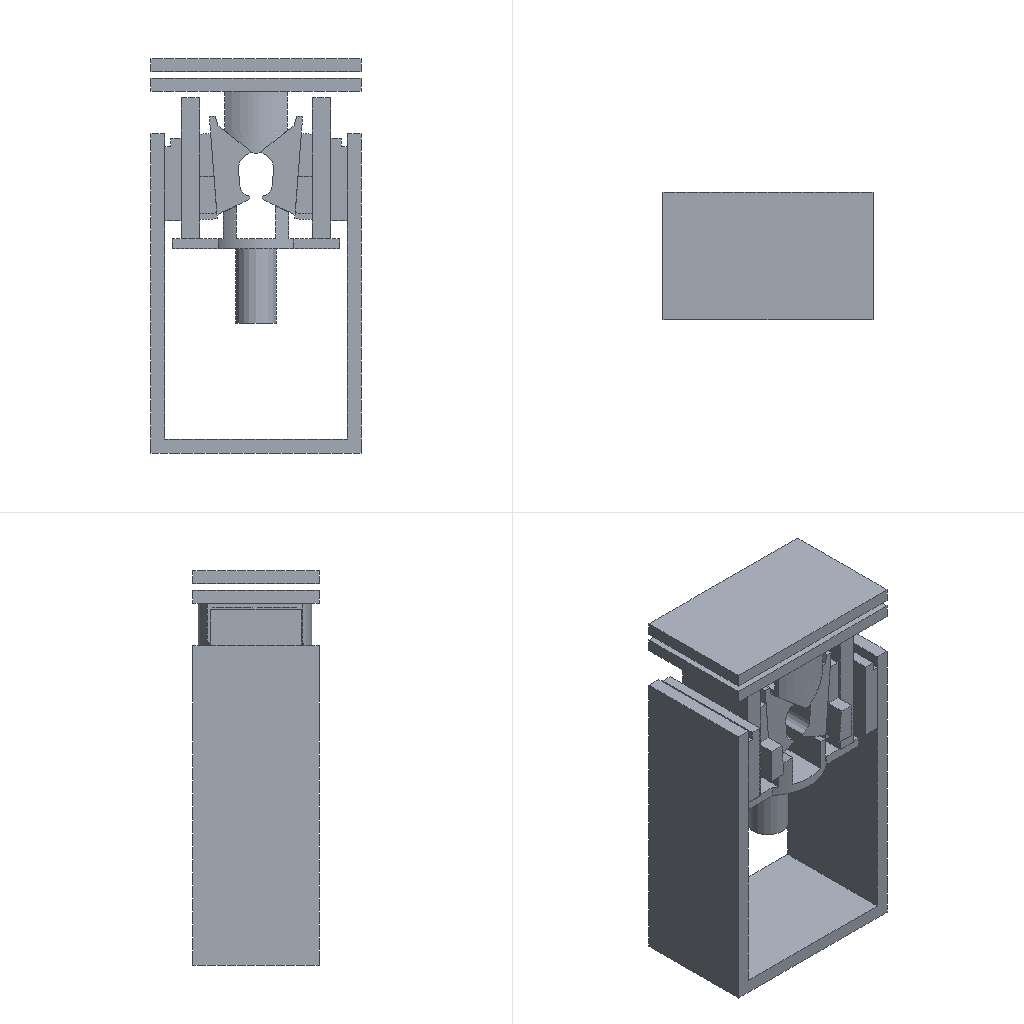Simulation study | abaqus
Set-up summary:
category,name,step,type,value,unit,region
solver,abaqus,,Abaqus/CAE 2024
units,mm-N-s-tonne (MPa),,inferred,E=212000 density=7.86e-09
analysis,Step-1,,dynamic temp-displacement,nlgeom=True; time_period=0.01
mesh,nodes,,,64430
mesh,elements,,,47881
element_type,C3D8T,,,47876
element_type,MASS,,,3
element_type,CONN3D2,,,2
material,hcq,,E,212000
material,hcq,,nu,0.3
material,hcq,,density,7.86e-09
material,hcq,,yield,400
material,hcq,,conductivity,50
material,hcq,,specific_heat,9.6e+08
material,hcq,,cte,1e-05
material,hcq,,behaviors,plastic; conductivity; expansion; specific heat
section,hcq,,solid section,,,Set-3
section,hcq,,solid section,,,Set-9
section,hcq,,solid section,,,Set-6
section,hcq,,solid section,,,Set-14
section,hcq,,solid section,,,Set-1
section,hcq,,solid section,,,Set-4
section,hcq,,solid section,,,Set-1
section,hcq,,solid section,,,Set-1
section,hcq,,solid section,,,Set-2
load,Predefined,initial,initial condition temperature
bc,BC-2,initial,encastre,[dofs=ENCASTRE],,Set-15
bc,BC-1,Step-1,velocity,"-2000 [dofs=x,y,z n=3]",,Set-5
contact,Constraint-2,initial,tie,,,s_Surf-17 / m_Surf-17
contact,Constraint-3,initial,tie,,,s_Surf-19 / m_Surf-19
contact,Constraint-4,initial,tie,,,s_Surf-21 / m_Surf-21
contact,Int-9,initial,general contact,interaction=IntProp-1; friction=0.3; behavior=hard
constraint,connector section,,,2
constraint,coupling,,,3
Abaqus input file, long lists of numbers shortened:
*Heading
** Job name: deck Model name: Model-1-Copy-Copy
** Generated by: Abaqus/CAE 2024
*Preprint, echo=NO, model=NO, history=NO, contact=NO
**
** PARTS
**
*Part, name=dongaban
*Node
      1,         -70.,        107.5,           0.
      2,         -70.,   99.537,           0.
** (2658 more lines like these left out)
*Element, type=C3D8T
   1,  141,  142,  170,  169,    1,    2,   30,   29
   2,  142,  143,  171,  170,    2,    3,   31,   30
** (1942 more lines like these left out)
*Nset, nset=Set-3, generate
    1,  2660,     1
*Elset, elset=Set-3, generate
    1,  1944,     1
** Section: Section-1
*Solid Section, elset=Set-3, material=hcq
,
*End Part
**
*Part, name=gudingxieban
*Node
      1,          94.,         -28.,         13.5
      2,          94.,         -28.,         24.5
** (6109 more lines like these left out)
*Element, type=C3D8T
  1,  214, 1306, 3776, 1084,    1,   55,  940,   68
  2, 1306, 1307, 3777, 3776,   55,   56,  941,  940
** (4846 more lines like these left out)
*Nset, nset=Set-9, generate
    1,  6111,     1
*Elset, elset=Set-9, generate
    1,  4848,     1
** Section: Section-1
*Solid Section, elset=Set-9, material=hcq
,
*End Part
**
*Part, name=tanhuangzuo
*Node
      1,   -83.442,           0.,          30.
      2,   -83.442,          15.,          30.
** (9119 more lines like these left out)
*Element, type=C3D8T
  1,  143, 1319, 5444, 1193,    1,   87, 1157,  108
  2, 1319, 1320, 5445, 5444,   87,   88, 1158, 1157
** (6650 more lines like these left out)
*Nset, nset=Set-6, generate
    1,  9121,     1
*Elset, elset=Set-6, generate
    1,  6652,     1
** Section: Section-1
*Solid Section, elset=Set-6, material=hcq
,
*End Part
**
*Part, name=waigudingban
*Node
      1,           7.,           0.,          18.
      2,           7.,         -35.,          18.
** (6070 more lines like these left out)
*Element, type=C3D8T
 1,  183, 1581, 1593,  182,    1,  157,  168,    4
 2, 1581, 1582, 1594, 1593,  157,  158,  167,  168
** (4610 more lines like these left out)
*Nset, nset=Set-14, generate
    1,  6072,     1
*Elset, elset=Set-14, generate
    1,  4612,     1
** Section: Section-1
*Solid Section, elset=Set-14, material=hcq
,
*End Part
**
*Part, name=xiangti
*Node
      1,         139.,        -96.5,          22.
      2,         139.,        -96.5,         487.
** (7618 more lines like these left out)
*Element, type=C3D8T
   1,  282, 2429, 5443, 2393,    1,   25,  737,  152
   2, 2429, 2430, 5444, 5443,   25,   26,  738,  737
** (4786 more lines like these left out)
*Node
   7621,           0.,           0.,          22.
*Nset, nset=xiangti-RefPt_, internal
7621,
*Nset, nset=Set-1, generate
    1,  7620,     1
*Elset, elset=Set-1, generate
    1,  4788,     1
** Section: Section-1
*Solid Section, elset=Set-1, material=hcq
,
*End Part
**
*Part, name=xiekuai
*Node
      1,           0.,           0.,         130.
      2,   19.199,  -50.074,         130.
** (4966 more lines like these left out)
*Element, type=C3D8T
   1,    3,    2,    5,    4,  219,  218,  221,  220
   2,    5,    2,   27,   75,  221,  218,  243,  291
** (3980 more lines like these left out)
*Nset, nset=Set-4, generate
    1,  4968,     1
*Elset, elset=Set-4, generate
    1,  3982,     1
** Section: Section-1
*Solid Section, elset=Set-4, material=hcq
,
*End Part
**
*Part, name=yali
*Node
      1,        -290.,         -20.,          20.
      2,        -290.,  -9.842,          20.
** (1978 more lines like these left out)
*Element, type=C3D8T
   1,   61,   62,   82,   81,    1,    2,   22,   21
   2,   62,   63,   83,   82,    2,    3,   23,   22
** (1214 more lines like these left out)
*Nset, nset=Set-1, generate
    1,  1980,     1
*Elset, elset=Set-1, generate
    1,  1216,     1
** Section: Section-1
*Solid Section, elset=Set-1, material=hcq
,
*End Part
**
*Part, name=yuyaban
*Node
      1,        -290.,         -20.,          20.
      2,        -290.,  -9.842,          20.
** (1978 more lines like these left out)
*Element, type=C3D8T
   1,   61,   62,   82,   81,    1,    2,   22,   21
   2,   62,   63,   83,   82,    2,    3,   23,   22
** (1214 more lines like these left out)
*Nset, nset=Set-1, generate
    1,  1980,     1
*Elset, elset=Set-1, generate
    1,  1216,     1
** Section: Section-1
*Solid Section, elset=Set-1, material=hcq
,
*End Part
**
*Part, name=zhongxinxiekuai
*Node
      1,         12.5,         72.5,          52.
      2,         12.5,         72.5,          60.
** (4102 more lines like these left out)
*Element, type=C3D8T
 1,    1,  109,  797,  114,  123,  809, 2369,  801
 2,  109,    2,  110,  797,  809,  127,  805, 2369
** (3230 more lines like these left out)
*Nset, nset=Set-2, generate
    1,  4104,     1
*Elset, elset=Set-2, generate
    1,  3232,     1
** Section: Section-1
*Solid Section, elset=Set-2, material=hcq
,
*End Part
**
**
** ASSEMBLY
**
*Assembly, name=Assembly
**
*Instance, name=zhongxinxiekuai, part=zhongxinxiekuai
12.272, 24.554, 794.895
12.272, 24.554, 794.895, 12.272, 25.554, 794.895,         180.
*End Instance
**
*Instance, name=xiekuai, part=xiekuai
-47.226, 87.606, 606.989
-47.226, 87.606, 606.989, -47.774, 88.197, 606.397, 237.425
*End Instance
**
*Instance, name=gudingxieban, part=gudingxieban
-75.15, 22.606, 636.723
-75.15, 22.606, 636.723, -75.72, 23.176, 636.131, 118.737
*End Instance
**
*Instance, name=dongban, part=dongaban
-101.728, 22.606,         678.
-101.728, 22.606,         678., -101.151, 23.183, 678.577,         120.
*End Instance
**
*Instance, name=xiekuai1, part=xiekuai
71.769, -42.394, 606.989
71.769, -42.394, 606.989, 71.162, -42.956, 606.427, 117.49
*End Instance
**
*Instance, name=waigudingban1, part=waigudingban
126.272, 22.606,        660.5
126.272, 22.606,        660.5, 125.694, 23.183, 659.923,         120.
*End Instance
**
*Instance, name=gudingxieban1, part=gudingxieban
72.714, 22.606, 637.761
72.714, 22.606, 637.761, 73.298, 22.021, 638.323, 238.72
*End Instance
**
*Instance, name=dongaban1, part=dongaban
98.272, 22.606,         678.
98.272, 22.606,         678., 98.849, 23.183, 678.577,         120.
*End Instance
**
*Instance, name=tanhuangzuo, part=tanhuangzuo
12.272, 22.606,        555.5
12.272, 22.606,        555.5, 12.849, 23.183, 556.077,         120.
*End Instance
**
*Instance, name=xiangti, part=xiangti
12.272, 22.606,        243.5
*End Instance
**
*Instance, name=waigudingban, part=waigudingban
-101.728, 22.606,        660.5
-101.728, 22.606,        660.5, -101.151, 23.183, 659.923,         240.
*End Instance
**
*Instance, name=yuyaban-1, part=yuyaban
142.272, -53.894, 794.895
*End Instance
**
*Instance, name=yali-1, part=yali
142.272, -53.894, 824.895
*End Instance
**
*Node
      1,   12.272,   22.606,   699.895
*Node
      2,   12.272,   22.606,        570.5
*Element, type=CONN3D2
4, 1, 2
*Connector Section, elset=_PickedSet114, behavior=ConnSect-2
Translator,
"Datum csys-2",
*Element, type=CONN3D2
5, 2, xiangti0.7621
*Connector Section, elset=_PickedSet117, behavior=ConnSect-1
Translator,
"Datum csys-2",
*Nset, nset=Set-1, instance=zhongxinxiekuai, generate
    1,  4104,     1
*Nset, nset=Set-1, instance=xiekuai, generate
    1,  4968,     1
*Nset, nset=Set-1, instance=dongban, generate
    1,  2660,     1
*Nset, nset=Set-1, instance=gudingxieban1, generate
    1,  6111,     1
*Nset, nset=Set-1, instance=xiekuai1, generate
    1,  4968,     1
*Nset, nset=Set-1, instance=tanhuangzuo, generate
    1,  9121,     1
*Nset, nset=Set-1, instance=gudingxieban, generate
    1,  6111,     1
*Nset, nset=Set-1, instance=dongaban1, generate
    1,  2660,     1
*Nset, nset=Set-1, instance=waigudingban1, generate
    1,  6072,     1
*Nset, nset=Set-1, instance=xiangti, generate
    1,  7620,     1
*Elset, elset=Set-1, instance=zhongxinxiekuai, generate
    1,  3232,     1
*Elset, elset=Set-1, instance=xiekuai, generate
    1,  3982,     1
*Elset, elset=Set-1, instance=dongban, generate
    1,  1944,     1
*Elset, elset=Set-1, instance=gudingxieban1, generate
    1,  4848,     1
*Elset, elset=Set-1, instance=xiekuai1, generate
    1,  3982,     1
*Elset, elset=Set-1, instance=tanhuangzuo, generate
    1,  6652,     1
*Elset, elset=Set-1, instance=gudingxieban, generate
    1,  4848,     1
*Elset, elset=Set-1, instance=dongaban1, generate
    1,  1944,     1
*Elset, elset=Set-1, instance=waigudingban1, generate
    1,  4612,     1
*Elset, elset=Set-1, instance=xiangti, generate
    1,  4788,     1
*Nset, nset=Set-4, instance=zhongxinxiekuai
   84,   85,   86,   87,   88,   89,   90,   91,   92,   93,   94,   95,   96,   98,   99,  100
  101,  102,  103,  104,  557,  558,  559,  560,  561,  562,  563,  567,  568,  569,  570,  571
** (15 more lines like these left out)
*Elset, elset=Set-4, instance=zhongxinxiekuai
 1032, 1033, 1034, 1035, 1036, 1037, 1038, 1039, 1048, 1049, 1050, 1051, 1052, 1053, 1054, 1055
 1064, 1065, 1066, 1067, 1068, 1069, 1070, 1071, 1072, 1073, 1074, 1075, 1076, 1077, 1078, 1079
** (13 more lines like these left out)
*Nset, nset=Set-5, instance=yali-1
    1,    2,    3,    4,    5,    6,    7,    8,    9,   10,   11,   12,   13,   14,   15,   16
   17,   18,   19,   20,   61,   62,   63,   64,   65,   66,   67,   68,   69,   70,   71,   72
** (40 more lines like these left out)
*Elset, elset=Set-5, instance=yali-1
    1,    2,    3,    4,    5,    6,    7,    8,    9,   10,   11,   12,   13,   14,   15,   16
   17,   18,   19,   39,   40,   41,   42,   43,   44,   45,   46,   47,   48,   49,   50,   51
** (36 more lines like these left out)
*Nset, nset=Set-7, instance=zhongxinxiekuai, generate
    1,  4104,     1
*Nset, nset=Set-7, instance=xiekuai, generate
    1,  4968,     1
*Nset, nset=Set-7, instance=dongban, generate
    1,  2660,     1
*Nset, nset=Set-7, instance=gudingxieban1, generate
    1,  6111,     1
*Nset, nset=Set-7, instance=xiekuai1, generate
    1,  4968,     1
*Nset, nset=Set-7, instance=tanhuangzuo, generate
    1,  9121,     1
*Nset, nset=Set-7, instance=yali-1, generate
    1,  1980,     1
*Nset, nset=Set-7, instance=gudingxieban, generate
    1,  6111,     1
*Nset, nset=Set-7, instance=dongaban1, generate
    1,  2660,     1
*Nset, nset=Set-7, instance=waigudingban1, generate
    1,  6072,     1
*Nset, nset=Set-7, instance=xiangti, generate
    1,  7620,     1
*Nset, nset=Set-7, instance=yuyaban-1, generate
    1,  1980,     1
*Nset, nset=Set-7, instance=waigudingban, generate
    1,  6072,     1
*Elset, elset=Set-7, instance=zhongxinxiekuai, generate
    1,  3232,     1
*Elset, elset=Set-7, instance=xiekuai, generate
    1,  3982,     1
*Elset, elset=Set-7, instance=dongban, generate
    1,  1944,     1
*Elset, elset=Set-7, instance=gudingxieban1, generate
    1,  4848,     1
*Elset, elset=Set-7, instance=xiekuai1, generate
    1,  3982,     1
*Elset, elset=Set-7, instance=tanhuangzuo, generate
    1,  6652,     1
*Elset, elset=Set-7, instance=yali-1, generate
    1,  1216,     1
*Elset, elset=Set-7, instance=gudingxieban, generate
    1,  4848,     1
*Elset, elset=Set-7, instance=dongaban1, generate
    1,  1944,     1
*Elset, elset=Set-7, instance=waigudingban1, generate
    1,  4612,     1
*Elset, elset=Set-7, instance=xiangti, generate
    1,  4788,     1
*Elset, elset=Set-7, instance=yuyaban-1, generate
    1,  1216,     1
*Elset, elset=Set-7, instance=waigudingban, generate
    1,  4612,     1
*Nset, nset=Set-15, instance=xiangti
    5,    6,    7,    8,    9,   10,   11,   12,   15,   16,   17,   18,   19,   20,   21,   22
  153,  154,  155,  156,  157,  158,  159,  160,  161,  162,  163,  164,  165,  166,  167,  168
** (162 more lines like these left out)
*Elset, elset=Set-15, instance=xiangti
  894,  895,  896,  897,  898,  899,  900,  901,  902,  903,  904,  905,  906,  907,  908,  909
  910,  911,  912,  913,  914,  915,  916,  917,  918,  919,  920,  921,  922,  923,  924,  925
** (150 more lines like these left out)
*Nset, nset=Set-16, instance=zhongxinxiekuai, generate
    1,  4104,     1
*Nset, nset=Set-16, instance=xiekuai, generate
    1,  4968,     1
*Nset, nset=Set-16, instance=dongban, generate
    1,  2660,     1
*Nset, nset=Set-16, instance=gudingxieban1, generate
    1,  6111,     1
*Nset, nset=Set-16, instance=xiekuai1, generate
    1,  4968,     1
*Nset, nset=Set-16, instance=tanhuangzuo, generate
    1,  9121,     1
*Nset, nset=Set-16, instance=yali-1, generate
    1,  1980,     1
*Nset, nset=Set-16, instance=gudingxieban, generate
    1,  6111,     1
*Nset, nset=Set-16, instance=dongaban1, generate
    1,  2660,     1
*Nset, nset=Set-16, instance=waigudingban1, generate
    1,  6072,     1
*Nset, nset=Set-16, instance=xiangti, generate
    1,  7620,     1
*Nset, nset=Set-16, instance=yuyaban-1, generate
    1,  1980,     1
*Nset, nset=Set-16, instance=waigudingban, generate
    1,  6072,     1
*Elset, elset=Set-16, instance=zhongxinxiekuai, generate
    1,  3232,     1
*Elset, elset=Set-16, instance=xiekuai, generate
    1,  3982,     1
*Elset, elset=Set-16, instance=dongban, generate
    1,  1944,     1
*Elset, elset=Set-16, instance=gudingxieban1, generate
    1,  4848,     1
*Elset, elset=Set-16, instance=xiekuai1, generate
    1,  3982,     1
*Elset, elset=Set-16, instance=tanhuangzuo, generate
    1,  6652,     1
*Elset, elset=Set-16, instance=yali-1, generate
    1,  1216,     1
*Elset, elset=Set-16, instance=gudingxieban, generate
    1,  4848,     1
*Elset, elset=Set-16, instance=dongaban1, generate
    1,  1944,     1
*Elset, elset=Set-16, instance=waigudingban1, generate
    1,  4612,     1
*Elset, elset=Set-16, instance=xiangti, generate
    1,  4788,     1
*Elset, elset=Set-16, instance=yuyaban-1, generate
    1,  1216,     1
*Elset, elset=Set-16, instance=waigudingban, generate
    1,  4612,     1
*Nset, nset=Wire-1-Set-1
 1, 2
*Elset, elset=Wire-1-Set-1
 4,
*Nset, nset=Wire-2-Set-1
 2,
*Nset, nset=Wire-2-Set-1, instance=xiangti
 7621,
*Elset, elset=Wire-2-Set-1
 5,
*Nset, nset=b_Set-2, instance=xiangti, generate
    1,  7620,     1
*Elset, elset=b_Set-2, instance=xiangti, generate
    1,  4788,     1
*Nset, nset=m_Set-6, instance=zhongxinxiekuai, generate
   1,  108,    1
*Nset, nset=m_Set-6, instance=xiekuai
    1,    2,    5,    8,    9,   13,   16,   17,   18,   19, 4753, 4754, 4757, 4760, 4761, 4765
 4768, 4769, 4770, 4771
*Nset, nset=m_Set-6, instance=dongban
    1,   28,  113,  140, 2521, 2548, 2633, 2660
*Nset, nset=m_Set-6, instance=gudingxieban1, generate
  1,  54,   1
*Nset, nset=m_Set-6, instance=xiekuai1
    1,    2,    5,    8,    9,   13,   16,   17,   18,   19, 4753, 4754, 4757, 4760, 4761, 4765
 4768, 4769, 4770, 4771
*Nset, nset=m_Set-6, instance=tanhuangzuo, generate
  1,  86,   1
*Nset, nset=m_Set-6, instance=yali-1
    1,   20,   41,   60, 1921, 1940, 1961, 1980
*Nset, nset=m_Set-6, instance=gudingxieban, generate
  1,  54,   1
*Nset, nset=m_Set-6, instance=dongaban1
    1,   28,  113,  140, 2521, 2548, 2633, 2660
*Nset, nset=m_Set-6, instance=waigudingban1, generate
   1,  156,    1
*Nset, nset=m_Set-6, instance=xiangti, generate
  1,  24,   1
*Nset, nset=m_Set-6, instance=yuyaban-1
    1,   20,   41,   60, 1921, 1940, 1961, 1980
*Nset, nset=m_Set-6, instance=waigudingban, generate
   1,  156,    1
*Nset, nset=m_Set-12, instance=xiangti
 7621,
*Nset, nset=m_Set-13
 2,
*Nset, nset=m_Set-15
 1,
*Nset, nset=s_Set-13, instance=tanhuangzuo
  5,  8,  9, 10, 14, 18, 57, 62
*Elset, elset=_PickedSet114, internal
 4,
*Elset, elset=_PickedSet117, internal
 5,
*Elset, elset=_m_Surf-1_S5, internal, instance=dongaban1
   82,   83,   84,   85,   86,   87,   88,   89,   90,   91,   92,   93,   94,   95,   96,   97
   98,   99,  100,  101,  102,  103,  104,  105,  106,  107,  108,  190,  191,  192,  193,  194
** (29 more lines like these left out)
*Surface, type=ELEMENT, name=m_Surf-1
_m_Surf-1_S5, S5
*Elset, elset=_m_Surf-3_S3, internal, instance=dongaban1
    1,    2,    3,    4,    5,    6,    7,    8,    9,   10,   11,   12,   13,   14,   15,   16
   17,   18,   19,   20,   21,   22,   23,   24,   25,   26,   27,  109,  110,  111,  112,  113
** (29 more lines like these left out)
*Surface, type=ELEMENT, name=m_Surf-3
_m_Surf-3_S3, S3
*Elset, elset=_m_Surf-5_S3, internal, instance=dongban
    1,    2,    3,    4,    5,    6,    7,    8,    9,   10,   11,   12,   13,   14,   15,   16
   17,   18,   19,   20,   21,   22,   23,   24,   25,   26,   27,  109,  110,  111,  112,  113
** (29 more lines like these left out)
*Surface, type=ELEMENT, name=m_Surf-5
_m_Surf-5_S3, S3
*Elset, elset=_m_Surf-7_S5, internal, instance=dongban
   82,   83,   84,   85,   86,   87,   88,   89,   90,   91,   92,   93,   94,   95,   96,   97
   98,   99,  100,  101,  102,  103,  104,  105,  106,  107,  108,  190,  191,  192,  193,  194
** (29 more lines like these left out)
*Surface, type=ELEMENT, name=m_Surf-7
_m_Surf-7_S5, S5
*Elset, elset=_m_Surf-9_S5, internal, instance=xiekuai1
    4,    6,   20,   21,   26,   33,   35,   38,   41,   53,   57,  185,  187,  201,  202,  207
  214,  216,  219,  222,  234,  238,  366,  368,  382,  383,  388,  395,  397,  400,  403,  415
** (14 more lines like these left out)
*Elset, elset=_m_Surf-9_S3, internal, instance=xiekuai1
    5,   28,   30,   31,   36,   42,   44,   46,   49,   61,   64,   71,   73,   76,  186,  209
  211,  212,  217,  223,  225,  227,  230,  242,  245,  252,  254,  257,  367,  390,  392,  393
** (18 more lines like these left out)
*Surface, type=ELEMENT, name=m_Surf-9
_m_Surf-9_S5, S5
_m_Surf-9_S3, S3
*Elset, elset=_m_Surf-11_S4, internal, instance=xiekuai1
    9,   22,   68,   83,   84,  190,  203,  249,  264,  265,  371,  384,  430,  445,  446,  552
  565,  611,  626,  627,  733,  746,  792,  807,  808,  914,  927,  973,  988,  989, 1095, 1108
** (5 more lines like these left out)
*Elset, elset=_m_Surf-11_S3, internal, instance=xiekuai1, generate
   23,  3824,   181
*Elset, elset=_m_Surf-11_S6, internal, instance=xiekuai1
   25,   69,   70,   91,  206,  250,  251,  272,  387,  431,  432,  453,  568,  612,  613,  634
  749,  793,  794,  815,  930,  974,  975,  996, 1111, 1155, 1156, 1177, 1292, 1336, 1337, 1358
** (4 more lines like these left out)
*Surface, type=ELEMENT, name=m_Surf-11
_m_Surf-11_S4, S4
_m_Surf-11_S3, S3
_m_Surf-11_S6, S6
*Elset, elset=_m_Surf-13_S3, internal, instance=zhongxinxiekuai
 1582, 1662, 1666, 1670, 1674, 1678, 1682, 1686, 1819, 1899, 1903, 1907, 1911, 1915, 1919, 1923
 2056, 2136, 2140, 2144, 2148, 2152, 2156, 2160, 2293, 2373, 2377, 2381, 2385, 2389, 2393, 2397
** (2 more lines like these left out)
*Elset, elset=_m_Surf-13_S5, internal, instance=zhongxinxiekuai
 1690, 1697, 1701, 1705, 1709, 1713, 1717, 1721, 1725, 1927, 1934, 1938, 1942, 1946, 1950, 1954
 1958, 1962, 2164, 2171, 2175, 2179, 2183, 2187, 2191, 2195, 2199, 2401, 2408, 2412, 2416, 2420
** (2 more lines like these left out)
*Surface, type=ELEMENT, name=m_Surf-13
_m_Surf-13_S3, S3
_m_Surf-13_S5, S5
*Elset, elset=_m_Surf-15_S5, internal, instance=xiekuai
    4,    6,   20,   21,   26,   33,   35,   38,   41,   53,   57,  185,  187,  201,  202,  207
  214,  216,  219,  222,  234,  238,  366,  368,  382,  383,  388,  395,  397,  400,  403,  415
** (14 more lines like these left out)
*Elset, elset=_m_Surf-15_S3, internal, instance=xiekuai
    5,   28,   30,   31,   36,   42,   44,   46,   49,   61,   64,   71,   73,   76,  186,  209
  211,  212,  217,  223,  225,  227,  230,  242,  245,  252,  254,  257,  367,  390,  392,  393
** (18 more lines like these left out)
*Surface, type=ELEMENT, name=m_Surf-15
_m_Surf-15_S5, S5
_m_Surf-15_S3, S3
*Elset, elset=_m_Surf-17_S5, internal, instance=yuyaban-1
   20,   21,   22,   23,   24,   25,   26,   27,   28,   29,   30,   31,   32,   33,   34,   35
   36,   37,   38,   58,   59,   60,   61,   62,   63,   64,   65,   66,   67,   68,   69,   70
** (36 more lines like these left out)
*Surface, type=ELEMENT, name=m_Surf-17
_m_Surf-17_S5, S5
*Elset, elset=_m_Surf-19_S1, internal, instance=xiangti, generate
 3896,  4788,     1
*Surface, type=ELEMENT, name=m_Surf-19
_m_Surf-19_S1, S1
*Elset, elset=_m_Surf-21_S2, internal, instance=xiangti, generate
   1,  893,    1
*Surface, type=ELEMENT, name=m_Surf-21
_m_Surf-21_S2, S2
*Elset, elset=_s_Surf-1_S5, internal, instance=waigudingban1
  262,  263,  264,  271,  272,  273,  280,  281,  282,  996,  997,  998, 1005, 1006, 1007, 1014
 1015, 1016, 1023, 1024, 1025, 1032, 1033, 1034, 1041, 1042, 1043, 1050, 1051, 1052, 1059, 1060
** (11 more lines like these left out)
*Elset, elset=_s_Surf-1_S6, internal, instance=waigudingban1
   49,   52,   55,   58,   61,   64,   67,   70,   73,   76,   79,   82,   85,   88,   91,   94
   97,  100,  103,  106,  109,  112,  115,  118,  121,  124,  127,  130,  133,  136,  139,  142
** (27 more lines like these left out)
*Elset, elset=_s_Surf-1_S4, internal, instance=waigudingban1
 1373, 1376, 1379, 1382, 1385, 1388, 1391, 1394, 1397, 1400, 1403, 1406, 1409, 1412, 1415, 1418
 1421, 1424, 1427, 1430, 1433, 1436, 1439, 1442, 1445, 1448, 1451, 1454, 1457, 1460, 1883, 1886
** (21 more lines like these left out)
*Surface, type=ELEMENT, name=s_Surf-1
_s_Surf-1_S5, S5
_s_Surf-1_S6, S6
_s_Surf-1_S4, S4
*Elset, elset=_s_Surf-3_S4, internal, instance=gudingxieban1
    3,    6,    9,   12,   15,   18,   21,   24,   27,   30,   33,   36,   39,   42,   45,   48
   51,   54,   57,   60,   63,   66,   69,   72,   75,   78,   81,   84,   87,   90,   93,   96
** (13 more lines like these left out)
*Elset, elset=_s_Surf-3_S6, internal, instance=gudingxieban1, generate
 3781,  4006,     3
*Elset, elset=_s_Surf-3_S5, internal, instance=gudingxieban1
 1601, 1602, 1607, 1608, 1613, 1614, 1619, 1620, 1625, 1626, 1631, 1632, 1637, 1638, 1643, 1644
 1649, 1650, 1655, 1656, 1661, 1662, 1667, 1668, 1673, 1674, 1679, 1680, 1685, 1686, 1691, 1692
** (30 more lines like these left out)
*Surface, type=ELEMENT, name=s_Surf-3
_s_Surf-3_S4, S4
_s_Surf-3_S6, S6
_s_Surf-3_S5, S5
*Elset, elset=_s_Surf-5_S5, internal, instance=waigudingban
  262,  263,  264,  271,  272,  273,  280,  281,  282,  996,  997,  998, 1005, 1006, 1007, 1014
 1015, 1016, 1023, 1024, 1025, 1032, 1033, 1034, 1041, 1042, 1043, 1050, 1051, 1052, 1059, 1060
** (11 more lines like these left out)
*Elset, elset=_s_Surf-5_S6, internal, instance=waigudingban
   49,   52,   55,   58,   61,   64,   67,   70,   73,   76,   79,   82,   85,   88,   91,   94
   97,  100,  103,  106,  109,  112,  115,  118,  121,  124,  127,  130,  133,  136,  139,  142
** (27 more lines like these left out)
*Elset, elset=_s_Surf-5_S4, internal, instance=waigudingban
 1373, 1376, 1379, 1382, 1385, 1388, 1391, 1394, 1397, 1400, 1403, 1406, 1409, 1412, 1415, 1418
 1421, 1424, 1427, 1430, 1433, 1436, 1439, 1442, 1445, 1448, 1451, 1454, 1457, 1460, 1883, 1886
** (21 more lines like these left out)
*Surface, type=ELEMENT, name=s_Surf-5
_s_Surf-5_S5, S5
_s_Surf-5_S6, S6
_s_Surf-5_S4, S4
*Elset, elset=_s_Surf-7_S5, internal, instance=gudingxieban
  465,  466,  467,  468,  477,  478,  479,  480,  489,  490,  491,  492,  501,  502,  503,  504
  513,  514,  515,  516,  525,  526,  527,  528,  537,  538,  539,  540,  549,  550,  551,  552
** (36 more lines like these left out)
*Elset, elset=_s_Surf-7_S2, internal, instance=gudingxieban
 1141, 1142, 1143, 1144, 1145, 1146, 1147, 1148, 1149, 1150, 1151, 1152, 1153, 1154, 1155, 1156
 1157, 1158, 1159, 1160, 1161, 1162, 1163, 1164, 1165, 1166, 1167, 1168, 1169, 1170, 1171, 1172
** (11 more lines like these left out)
*Surface, type=ELEMENT, name=s_Surf-7
_s_Surf-7_S5, S5
_s_Surf-7_S2, S2
*Elset, elset=_s_Surf-9_S5, internal, instance=gudingxieban1
  465,  466,  467,  468,  477,  478,  479,  480,  489,  490,  491,  492,  501,  502,  503,  504
  513,  514,  515,  516,  525,  526,  527,  528,  537,  538,  539,  540,  549,  550,  551,  552
** (36 more lines like these left out)
*Elset, elset=_s_Surf-9_S2, internal, instance=gudingxieban1
 1141, 1142, 1143, 1144, 1145, 1146, 1147, 1148, 1149, 1150, 1151, 1152, 1153, 1154, 1155, 1156
 1157, 1158, 1159, 1160, 1161, 1162, 1163, 1164, 1165, 1166, 1167, 1168, 1169, 1170, 1171, 1172
** (11 more lines like these left out)
*Surface, type=ELEMENT, name=s_Surf-9
_s_Surf-9_S5, S5
_s_Surf-9_S2, S2
*Elset, elset=_s_Surf-11_S4, internal, instance=zhongxinxiekuai
 1609, 1753, 1757, 1761, 1765, 1769, 1773, 1777, 1785, 1846, 1990, 1994, 1998, 2002, 2006, 2010
 2014, 2022, 2083, 2227, 2231, 2235, 2239, 2243, 2247, 2251, 2259, 2320, 2464, 2468, 2472, 2476
** (2 more lines like these left out)
*Elset, elset=_s_Surf-11_S6, internal, instance=zhongxinxiekuai
 1631, 1632, 1633, 1634, 1635, 1636, 1637, 1868, 1869, 1870, 1871, 1872, 1873, 1874, 2105, 2106
 2107, 2108, 2109, 2110, 2111, 2342, 2343, 2344, 2345, 2346, 2347, 2348, 2579, 2580, 2581, 2582
** (2 more lines like these left out)
*Elset, elset=_s_Surf-11_S3, internal, instance=zhongxinxiekuai, generate
 1778,  3200,   237
*Surface, type=ELEMENT, name=s_Surf-11
_s_Surf-11_S4, S4
_s_Surf-11_S6, S6
_s_Surf-11_S3, S3
*Elset, elset=_s_Surf-13_S4, internal, instance=xiekuai
    9,   22,   68,   83,   84,  190,  203,  249,  264,  265,  371,  384,  430,  445,  446,  552
  565,  611,  626,  627,  733,  746,  792,  807,  808,  914,  927,  973,  988,  989, 1095, 1108
** (5 more lines like these left out)
*Elset, elset=_s_Surf-13_S3, internal, instance=xiekuai, generate
   23,  3824,   181
*Elset, elset=_s_Surf-13_S6, internal, instance=xiekuai
   25,   69,   70,   91,  206,  250,  251,  272,  387,  431,  432,  453,  568,  612,  613,  634
  749,  793,  794,  815,  930,  974,  975,  996, 1111, 1155, 1156, 1177, 1292, 1336, 1337, 1358
** (4 more lines like these left out)
*Surface, type=ELEMENT, name=s_Surf-13
_s_Surf-13_S4, S4
_s_Surf-13_S3, S3
_s_Surf-13_S6, S6
*Elset, elset=_s_Surf-15_S4, internal, instance=gudingxieban
    3,    6,    9,   12,   15,   18,   21,   24,   27,   30,   33,   36,   39,   42,   45,   48
   51,   54,   57,   60,   63,   66,   69,   72,   75,   78,   81,   84,   87,   90,   93,   96
** (13 more lines like these left out)
*Elset, elset=_s_Surf-15_S6, internal, instance=gudingxieban, generate
 3781,  4006,     3
*Elset, elset=_s_Surf-15_S5, internal, instance=gudingxieban
 1601, 1602, 1607, 1608, 1613, 1614, 1619, 1620, 1625, 1626, 1631, 1632, 1637, 1638, 1643, 1644
 1649, 1650, 1655, 1656, 1661, 1662, 1667, 1668, 1673, 1674, 1679, 1680, 1685, 1686, 1691, 1692
** (30 more lines like these left out)
*Surface, type=ELEMENT, name=s_Surf-15
_s_Surf-15_S4, S4
_s_Surf-15_S6, S6
_s_Surf-15_S5, S5
*Elset, elset=_s_Surf-17_S3, internal, instance=zhongxinxiekuai
 1032, 1033, 1048, 1049, 1050, 1051, 1064, 1065, 1066, 1067, 1408, 1409
*Elset, elset=_s_Surf-17_S4, internal, instance=zhongxinxiekuai
 1034, 1035, 1036, 1037, 1052, 1053, 1068, 1069, 1155, 1157, 1159, 1161, 1163, 1165, 1167, 1169
 1171, 1173, 1175, 1177, 1179, 1181, 1183, 1185, 1187, 1189, 1191, 1193, 1195, 1197, 1199, 1201
** (3 more lines like these left out)
*Elset, elset=_s_Surf-17_S2, internal, instance=zhongxinxiekuai
 1038, 1039, 1054, 1055, 1070, 1071, 1072, 1073, 1074, 1075, 1076, 1077, 1078, 1079, 1080, 1202
 1203, 1204, 1205, 1206, 1207, 1208, 1209, 1210, 1211, 1212, 1213, 1214, 1215, 1216, 1217, 1218
** (4 more lines like these left out)
*Elset, elset=_s_Surf-17_S6, internal, instance=zhongxinxiekuai
 1090, 1092, 1094, 1096, 1098, 1100, 1102, 1104, 1106, 1108, 1110, 1112, 1114, 1116, 1118, 1120
 1122, 1124, 1126, 1128, 1130, 1132, 1134, 1136, 1138, 1140, 1142, 1144, 1146, 1148, 1150, 1152
** (2 more lines like these left out)
*Surface, type=ELEMENT, name=s_Surf-17
_s_Surf-17_S3, S3
_s_Surf-17_S4, S4
_s_Surf-17_S2, S2
_s_Surf-17_S6, S6
*Elset, elset=_s_Surf-19_S6, internal, instance=waigudingban
  292,  293,  294,  295,  296,  297,  298,  299,  300, 1086, 1087, 1088, 1089, 1090, 1091, 1092
 1093, 1094, 1095, 1096, 1097, 1098, 1099, 1100, 1101, 1102, 1103, 1104, 1105, 1106, 1107, 1108
** (6 more lines like these left out)
*Elset, elset=_s_Surf-19_S3, internal, instance=waigudingban
  301,  302,  303,  304,  305,  306,  307,  308,  309, 1110, 1111, 1112, 1113, 1114, 1115, 1116
 1117, 1118, 1119, 1120, 1121, 1122, 1123, 1124, 1125, 1126, 1127, 1128, 1129, 1130, 1131, 1132
** (3 more lines like these left out)
*Elset, elset=_s_Surf-19_S5, internal, instance=waigudingban
   31,   32,   33,   34,   35,   36,   37,   38,   39,  390,  391,  392,  393,  394,  395,  396
  397,  398,  399,  400,  401,  402,  403,  404,  405,  406,  407,  408,  409,  410,  411,  412
** (22 more lines like these left out)
*Elset, elset=_s_Surf-19_S4, internal, instance=waigudingban, generate
 2181,  2210,     1
*Elset, elset=_s_Surf-19_S2, internal, instance=waigudingban, generate
 4361,  4430,     1
*Surface, type=ELEMENT, name=s_Surf-19
_s_Surf-19_S6, S6
_s_Surf-19_S3, S3
_s_Surf-19_S4, S4
_s_Surf-19_S2, S2
_s_Surf-19_S5, S5
*Elset, elset=_s_Surf-21_S6, internal, instance=waigudingban1
  292,  293,  294,  295,  296,  297,  298,  299,  300, 1086, 1087, 1088, 1089, 1090, 1091, 1092
 1093, 1094, 1095, 1096, 1097, 1098, 1099, 1100, 1101, 1102, 1103, 1104, 1105, 1106, 1107, 1108
** (6 more lines like these left out)
*Elset, elset=_s_Surf-21_S3, internal, instance=waigudingban1
  301,  302,  303,  304,  305,  306,  307,  308,  309, 1110, 1111, 1112, 1113, 1114, 1115, 1116
 1117, 1118, 1119, 1120, 1121, 1122, 1123, 1124, 1125, 1126, 1127, 1128, 1129, 1130, 1131, 1132
** (3 more lines like these left out)
*Elset, elset=_s_Surf-21_S5, internal, instance=waigudingban1
   31,   32,   33,   34,   35,   36,   37,   38,   39,  390,  391,  392,  393,  394,  395,  396
  397,  398,  399,  400,  401,  402,  403,  404,  405,  406,  407,  408,  409,  410,  411,  412
** (22 more lines like these left out)
*Elset, elset=_s_Surf-21_S4, internal, instance=waigudingban1, generate
 2181,  2210,     1
*Elset, elset=_s_Surf-21_S2, internal, instance=waigudingban1, generate
 4361,  4430,     1
*Surface, type=ELEMENT, name=s_Surf-21
_s_Surf-21_S6, S6
_s_Surf-21_S3, S3
_s_Surf-21_S4, S4
_s_Surf-21_S2, S2
_s_Surf-21_S5, S5
*Elset, elset=_s_Surf-23_S1, internal, instance=xiangti, generate
 2395,  2926,     1
*Surface, type=ELEMENT, name=s_Surf-23
_s_Surf-23_S1, S1
*Elset, elset=_s_Surf-24_S2, internal, instance=xiangti, generate
 1863,  2394,     1
*Surface, type=ELEMENT, name=s_Surf-24
_s_Surf-24_S2, S2
*Elset, elset=_s_Surf-25_S2, internal, instance=zhongxinxiekuai, generate
 2996,  3232,     1
*Surface, type=ELEMENT, name=s_Surf-25
_s_Surf-25_S2, S2
*Surface, type=NODE, name=s_Set-13_CNS_, internal
s_Set-13, 1.
*Orientation, name="Datum csys-2"
          0.,           0.,           1.,           0.,           1.,           0.
1, 0.
** Constraint: Constraint-2
*Tie, name=Constraint-2, adjust=no
s_Surf-17, m_Surf-17
** Constraint: Constraint-3
*Tie, name=Constraint-3, adjust=no
s_Surf-19, m_Surf-19
** Constraint: Constraint-4
*Tie, name=Constraint-4, adjust=no
s_Surf-21, m_Surf-21
** Constraint: Constraint-5
*Coupling, constraint name=Constraint-5, ref node=m_Set-12, surface=s_Surf-24
*Kinematic
** Constraint: Constraint-6
*Coupling, constraint name=Constraint-6, ref node=m_Set-13, surface=s_Set-13_CNS_
*Kinematic
** Constraint: Constraint-7
*Coupling, constraint name=Constraint-7, ref node=m_Set-15, surface=s_Surf-25
*Kinematic
*Element, type=MASS, elset=_PickedSet110_Inertia-1_
1, xiangti0.7621
2, 1
** (1 more lines like these left out)
*Mass, elset=_PickedSet110_Inertia-1_
1e-06,
*End Assembly
*Connector Behavior, name=ConnSect-2
*Connector Elasticity, component=1
129.,
*Connector Behavior, name=ConnSect-1
*Connector Elasticity, component=1
1287.,
**
** MATERIALS
**
*Material, name=hcq
*Conductivity
50.,
*Density
 7.86e-09,
*Elastic
212000., 0.3
*Expansion
 1e-05,
*Plastic
400.,0.
*Specific Heat
 9.6e+08,
**
** INTERACTION PROPERTIES
**
*Surface Interaction, name=IntProp-1
*Friction
 0.3,
*Surface Behavior, pressure-overclosure=HARD
*Gap Heat Generation
1., 0.5
*Surface Interaction, name=IntProp-2
*Friction
 0.3,
*Surface Behavior, pressure-overclosure=HARD
**
** BOUNDARY CONDITIONS
**
** Name: BC-2 Type: Symmetry/Antisymmetry/Encastre
*Boundary
Set-15, ENCASTRE
**
** PREDEFINED FIELDS
**
** Name: Predefined Field-1   Type: Temperature
*Initial Conditions, type=TEMPERATURE
Set-16, 25.
**
** INTERACTIONS
**
** Interaction: Int-9
*Contact, op=NEW
*Contact Inclusions, ALL EXTERIOR
*Contact Property Assignment
 ,  , IntProp-1
** ----------------------------------------------------------------
**
** STEP: Step-1
**
*Step, name=Step-1, nlgeom=YES
*Dynamic Temperature-displacement, Explicit
, 0.01
*Bulk Viscosity
0.06, 1.2
** Mass Scaling: Semi-Automatic
**               Whole Model
*Fixed Mass Scaling, factor=1000.
**
** BOUNDARY CONDITIONS
**
** Name: BC-1 Type: Velocity/Angular velocity
*Boundary, type=VELOCITY
Set-5, 1, 1
Set-5, 2, 2
Set-5, 3, 3, -2000.
**
** OUTPUT REQUESTS
**
*Restart, write, number interval=1, time marks=NO
**
** FIELD OUTPUT: F-Output-1
**
*Output, field
*Node Output
A, NT, RF, RFL, U, V
*Element Output, directions=YES
EVF, HFL, LE, PE, PEEQ, PEEQVAVG, PEVAVG, S, SVAVG, TEMP
*Contact Output
CSTRESS,
**
** HISTORY OUTPUT: H-Output-1
**
*Output, history, variable=PRESELECT, frequency=1
*End Step
Results summary:
result,odb.job_status,,,JOB_STATUS_COMPLETED_SUCCESSFULLY,"consistent, unstated (Abaqus has no unit system)"
result,steps[0].procedure,Step-1,,"*DYNAMIC TEMPERATURE-DISPLACEMENT, EXPLICT","consistent, unstated (Abaqus has no unit system)"
result,steps[0].time_period,Step-1,,0.01,"consistent, unstated (Abaqus has no unit system)"
result,steps[0].n_frames,Step-1,,21,"consistent, unstated (Abaqus has no unit system)"
result,steps[0].last_frame.id,Step-1,,9575,"consistent, unstated (Abaqus has no unit system)"
result,steps[0].last_frame.value,Step-1,,0.01,"consistent, unstated (Abaqus has no unit system)"
result,steps[0].last_frame.description,Step-1,,Increment      9575: Step Time =   1.0000E-02,"consistent, unstated (Abaqus has no unit system)"
result,steps[0].completed,Step-1,,True,"consistent, unstated (Abaqus has no unit system)"
result,steps[0].max_U_magnitude,Step-1,,20.014,"consistent, unstated (Abaqus has no unit system)"
result,steps[0].max_S_mises,Step-1,,400.002,"consistent, unstated (Abaqus has no unit system)"
result,steps[0].RF_sum[1],Step-1,,34726.8,"consistent, unstated (Abaqus has no unit system)"
result,steps[0].RF_sum[2],Step-1,,23916,"consistent, unstated (Abaqus has no unit system)"
result,steps[0].RF_sum[3],Step-1,,192780,"consistent, unstated (Abaqus has no unit system)"
result,steps[0].diagnostic.n_increments,Step-1,,21,"consistent, unstated (Abaqus has no unit system)"